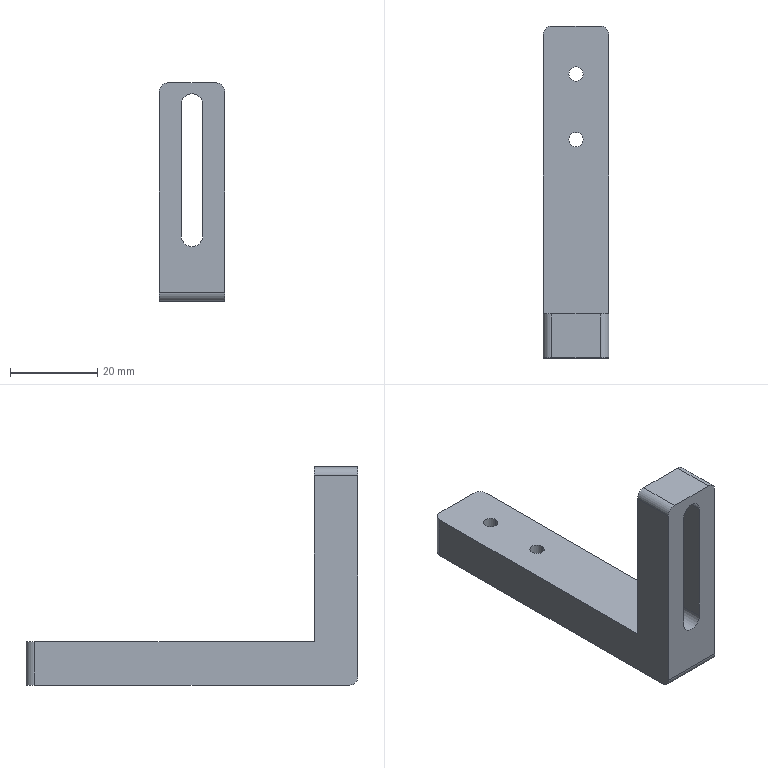Part | STEP file | 1004-2001-0086-1_1004-2001-0086-2 | 1 solid | 22 faces | box 15 x 76 x 50 mm | volume 15485 mm3 | cylinder 12 | plane 10 | commonest cylinder face diameters 4 x5 3.3 x4 5 x3
STEP:
#1=CARTESIAN_POINT('',(1.65,55.,-40.));
#2=VERTEX_POINT('',#1);
#3=CARTESIAN_POINT('',(-1.65,55.,-40.));
#4=VERTEX_POINT('',#3);
#5=CARTESIAN_POINT('',(0.,55.,-40.));
#6=DIRECTION('',(0.,0.,-1.));
#7=DIRECTION('',(-1.,0.,0.));
#8=AXIS2_PLACEMENT_3D('',#5,#6,#7);
#9=CIRCLE('',#8,1.65);
#10=EDGE_CURVE('',#2,#4,#9,.T.);
#11=ORIENTED_EDGE('',*,*,#10,.F.);
#12=CARTESIAN_POINT('',(1.65,55.,-50.));
#13=VERTEX_POINT('',#12);
#14=CARTESIAN_POINT('',(1.65,55.,-50.));
#15=DIRECTION('',(0.,0.,-1.));
#16=VECTOR('',#15,1000.);
#17=LINE('',#14,#16);
#18=EDGE_CURVE('',#2,#13,#17,.T.);
#19=ORIENTED_EDGE('',*,*,#18,.T.);
#20=CARTESIAN_POINT('',(-1.65,55.,-50.));
#21=VERTEX_POINT('',#20);
#22=CARTESIAN_POINT('',(0.,55.,-50.));
#23=DIRECTION('',(0.,0.,-1.));
#24=DIRECTION('',(-1.,0.,0.));
#25=AXIS2_PLACEMENT_3D('',#22,#23,#24);
#26=CIRCLE('',#25,1.65);
#27=EDGE_CURVE('',#13,#21,#26,.T.);
#28=ORIENTED_EDGE('',*,*,#27,.T.);
#29=CARTESIAN_POINT('',(-1.65,55.,-50.));
#30=DIRECTION('',(0.,0.,-1.));
#31=VECTOR('',#30,1000.);
#32=LINE('',#29,#31);
#33=EDGE_CURVE('',#4,#21,#32,.T.);
#34=ORIENTED_EDGE('',*,*,#33,.F.);
#35=EDGE_LOOP('',(#11,#19,#28,#34));
#36=FACE_OUTER_BOUND('',#35,.T.);
#37=CARTESIAN_POINT('',(0.,55.,-50.));
#38=DIRECTION('',(0.,0.,-1.));
#39=DIRECTION('',(-1.,0.,0.));
#40=AXIS2_PLACEMENT_3D('',#37,#38,#39);
#41=CYLINDRICAL_SURFACE('',#40,1.65);
#42=ADVANCED_FACE('',(#36),#41,.F.);
#43=CARTESIAN_POINT('',(1.65,40.,-40.));
#44=VERTEX_POINT('',#43);
#45=CARTESIAN_POINT('',(-1.65,40.,-40.));
#46=VERTEX_POINT('',#45);
#47=CARTESIAN_POINT('',(0.,40.,-40.));
#48=DIRECTION('',(0.,0.,-1.));
#49=DIRECTION('',(-1.,0.,0.));
#50=AXIS2_PLACEMENT_3D('',#47,#48,#49);
#51=CIRCLE('',#50,1.65);
#52=EDGE_CURVE('',#44,#46,#51,.T.);
#53=ORIENTED_EDGE('',*,*,#52,.F.);
#54=CARTESIAN_POINT('',(1.65,40.,-50.));
#55=VERTEX_POINT('',#54);
#56=CARTESIAN_POINT('',(1.65,40.,-50.));
#57=DIRECTION('',(0.,0.,-1.));
#58=VECTOR('',#57,1000.);
#59=LINE('',#56,#58);
#60=EDGE_CURVE('',#44,#55,#59,.T.);
#61=ORIENTED_EDGE('',*,*,#60,.T.);
#62=CARTESIAN_POINT('',(-1.65,40.,-50.));
#63=VERTEX_POINT('',#62);
#64=CARTESIAN_POINT('',(0.,40.,-50.));
#65=DIRECTION('',(0.,0.,-1.));
#66=DIRECTION('',(-1.,0.,0.));
#67=AXIS2_PLACEMENT_3D('',#64,#65,#66);
#68=CIRCLE('',#67,1.65);
#69=EDGE_CURVE('',#55,#63,#68,.T.);
#70=ORIENTED_EDGE('',*,*,#69,.T.);
#71=CARTESIAN_POINT('',(-1.65,40.,-50.));
#72=DIRECTION('',(0.,0.,-1.));
#73=VECTOR('',#72,1000.);
#74=LINE('',#71,#73);
#75=EDGE_CURVE('',#46,#63,#74,.T.);
#76=ORIENTED_EDGE('',*,*,#75,.F.);
#77=EDGE_LOOP('',(#53,#61,#70,#76));
#78=FACE_OUTER_BOUND('',#77,.T.);
#79=CARTESIAN_POINT('',(0.,40.,-50.));
#80=DIRECTION('',(0.,0.,-1.));
#81=DIRECTION('',(-1.,0.,0.));
#82=AXIS2_PLACEMENT_3D('',#79,#80,#81);
#83=CYLINDRICAL_SURFACE('',#82,1.65);
#84=ADVANCED_FACE('',(#78),#83,.F.);
#85=CARTESIAN_POINT('',(2.5,-10.,-5.));
#86=VERTEX_POINT('',#85);
#87=CARTESIAN_POINT('',(0.,-10.,-2.5));
#88=VERTEX_POINT('',#87);
#89=CARTESIAN_POINT('',(0.,-10.,-5.));
#90=DIRECTION('',(0.,-1.,0.));
#91=DIRECTION('',(0.,0.,1.));
#92=AXIS2_PLACEMENT_3D('',#89,#90,#91);
#93=CIRCLE('',#92,2.5);
#94=EDGE_CURVE('',#86,#88,#93,.T.);
#95=ORIENTED_EDGE('',*,*,#94,.T.);
#96=CARTESIAN_POINT('',(0.,0.,-2.5));
#97=VERTEX_POINT('',#96);
#98=CARTESIAN_POINT('',(0.,-10.,-2.5));
#99=DIRECTION('',(0.,1.,0.));
#100=VECTOR('',#99,1000.);
#101=LINE('',#98,#100);
#102=EDGE_CURVE('',#88,#97,#101,.T.);
#103=ORIENTED_EDGE('',*,*,#102,.T.);
#104=CARTESIAN_POINT('',(2.5,0.,-5.));
#105=VERTEX_POINT('',#104);
#106=CARTESIAN_POINT('',(0.,0.,-5.));
#107=DIRECTION('',(0.,-1.,0.));
#108=DIRECTION('',(0.,0.,1.));
#109=AXIS2_PLACEMENT_3D('',#106,#107,#108);
#110=CIRCLE('',#109,2.5);
#111=EDGE_CURVE('',#105,#97,#110,.T.);
#112=ORIENTED_EDGE('',*,*,#111,.F.);
#113=CARTESIAN_POINT('',(2.5,-10.,-5.));
#114=DIRECTION('',(0.,1.,0.));
#115=VECTOR('',#114,1000.);
#116=LINE('',#113,#115);
#117=EDGE_CURVE('',#86,#105,#116,.T.);
#118=ORIENTED_EDGE('',*,*,#117,.F.);
#119=EDGE_LOOP('',(#95,#103,#112,#118));
#120=FACE_OUTER_BOUND('',#119,.T.);
#121=CARTESIAN_POINT('',(0.,-10.,-5.));
#122=DIRECTION('',(0.,1.,0.));
#123=DIRECTION('',(0.,0.,1.));
#124=AXIS2_PLACEMENT_3D('',#121,#122,#123);
#125=CYLINDRICAL_SURFACE('',#124,2.5);
#126=ADVANCED_FACE('',(#120),#125,.F.);
#127=CARTESIAN_POINT('',(-7.5,64.,-40.));
#128=VERTEX_POINT('',#127);
#129=CARTESIAN_POINT('',(-7.5,64.,-50.));
#130=VERTEX_POINT('',#129);
#131=CARTESIAN_POINT('',(-7.5,64.,-50.));
#132=DIRECTION('',(0.,0.,-1.));
#133=VECTOR('',#132,1000.);
#134=LINE('',#131,#133);
#135=EDGE_CURVE('',#128,#130,#134,.T.);
#136=ORIENTED_EDGE('',*,*,#135,.T.);
#137=CARTESIAN_POINT('',(-7.5,-8.,-50.));
#138=VERTEX_POINT('',#137);
#139=CARTESIAN_POINT('',(-7.5,66.,-50.));
#140=DIRECTION('',(0.,-1.,0.));
#141=VECTOR('',#140,1000.);
#142=LINE('',#139,#141);
#143=EDGE_CURVE('',#130,#138,#142,.T.);
#144=ORIENTED_EDGE('',*,*,#143,.T.);
#145=CARTESIAN_POINT('',(-7.5,-10.,-48.));
#146=VERTEX_POINT('',#145);
#147=CARTESIAN_POINT('',(-7.5,-8.,-48.));
#148=DIRECTION('',(-1.,0.,0.));
#149=DIRECTION('',(0.,0.,1.));
#150=AXIS2_PLACEMENT_3D('',#147,#148,#149);
#151=CIRCLE('',#150,2.);
#152=EDGE_CURVE('',#138,#146,#151,.T.);
#153=ORIENTED_EDGE('',*,*,#152,.T.);
#154=CARTESIAN_POINT('',(-7.5,-10.,-2.));
#155=VERTEX_POINT('',#154);
#156=CARTESIAN_POINT('',(-7.5,-10.,-50.));
#157=DIRECTION('',(0.,0.,1.));
#158=VECTOR('',#157,1000.);
#159=LINE('',#156,#158);
#160=EDGE_CURVE('',#146,#155,#159,.T.);
#161=ORIENTED_EDGE('',*,*,#160,.T.);
#162=CARTESIAN_POINT('',(-7.5,0.,-2.));
#163=VERTEX_POINT('',#162);
#164=CARTESIAN_POINT('',(-7.5,66.,-2.));
#165=DIRECTION('',(0.,1.,0.));
#166=VECTOR('',#165,1000.);
#167=LINE('',#164,#166);
#168=EDGE_CURVE('',#155,#163,#167,.T.);
#169=ORIENTED_EDGE('',*,*,#168,.T.);
#170=CARTESIAN_POINT('',(-7.5,0.,-40.));
#171=VERTEX_POINT('',#170);
#172=CARTESIAN_POINT('',(-7.5,0.,-50.));
#173=DIRECTION('',(0.,0.,-1.));
#174=VECTOR('',#173,1000.);
#175=LINE('',#172,#174);
#176=EDGE_CURVE('',#163,#171,#175,.T.);
#177=ORIENTED_EDGE('',*,*,#176,.T.);
#178=CARTESIAN_POINT('',(-7.5,66.,-40.));
#179=DIRECTION('',(0.,1.,0.));
#180=VECTOR('',#179,1000.);
#181=LINE('',#178,#180);
#182=EDGE_CURVE('',#171,#128,#181,.T.);
#183=ORIENTED_EDGE('',*,*,#182,.T.);
#184=EDGE_LOOP('',(#136,#144,#153,#161,#169,#177,#183));
#185=FACE_OUTER_BOUND('',#184,.T.);
#186=CARTESIAN_POINT('',(-7.5,66.,-50.));
#187=DIRECTION('',(-1.,0.,0.));
#188=DIRECTION('',(0.,0.,1.));
#189=AXIS2_PLACEMENT_3D('',#186,#187,#188);
#190=PLANE('',#189);
#191=ADVANCED_FACE('',(#185),#190,.T.);
#192=CARTESIAN_POINT('',(0.,55.,-50.));
#193=DIRECTION('',(0.,0.,-1.));
#194=DIRECTION('',(-1.,0.,0.));
#195=AXIS2_PLACEMENT_3D('',#192,#193,#194);
#196=CIRCLE('',#195,1.65);
#197=EDGE_CURVE('',#21,#13,#196,.T.);
#198=ORIENTED_EDGE('',*,*,#197,.F.);
#199=ORIENTED_EDGE('',*,*,#27,.F.);
#200=EDGE_LOOP('',(#198,#199));
#201=FACE_BOUND('',#200,.T.);
#202=CARTESIAN_POINT('',(0.,40.,-50.));
#203=DIRECTION('',(0.,0.,-1.));
#204=DIRECTION('',(-1.,0.,0.));
#205=AXIS2_PLACEMENT_3D('',#202,#203,#204);
#206=CIRCLE('',#205,1.65);
#207=EDGE_CURVE('',#63,#55,#206,.T.);
#208=ORIENTED_EDGE('',*,*,#207,.F.);
#209=ORIENTED_EDGE('',*,*,#69,.F.);
#210=EDGE_LOOP('',(#208,#209));
#211=FACE_BOUND('',#210,.T.);
#212=ORIENTED_EDGE('',*,*,#143,.F.);
#213=CARTESIAN_POINT('',(-5.5,66.,-50.));
#214=VERTEX_POINT('',#213);
#215=CARTESIAN_POINT('',(-5.5,64.,-50.));
#216=DIRECTION('',(0.,0.,1.));
#217=DIRECTION('',(-1.,0.,0.));
#218=AXIS2_PLACEMENT_3D('',#215,#216,#217);
#219=CIRCLE('',#218,2.);
#220=EDGE_CURVE('',#214,#130,#219,.T.);
#221=ORIENTED_EDGE('',*,*,#220,.F.);
#222=CARTESIAN_POINT('',(5.5,66.,-50.));
#223=VERTEX_POINT('',#222);
#224=CARTESIAN_POINT('',(7.5,66.,-50.));
#225=DIRECTION('',(-1.,0.,0.));
#226=VECTOR('',#225,1000.);
#227=LINE('',#224,#226);
#228=EDGE_CURVE('',#223,#214,#227,.T.);
#229=ORIENTED_EDGE('',*,*,#228,.F.);
#230=CARTESIAN_POINT('',(7.5,64.,-50.));
#231=VERTEX_POINT('',#230);
#232=CARTESIAN_POINT('',(5.5,64.,-50.));
#233=DIRECTION('',(0.,0.,1.));
#234=DIRECTION('',(1.,0.,0.));
#235=AXIS2_PLACEMENT_3D('',#232,#233,#234);
#236=CIRCLE('',#235,2.);
#237=EDGE_CURVE('',#231,#223,#236,.T.);
#238=ORIENTED_EDGE('',*,*,#237,.F.);
#239=CARTESIAN_POINT('',(7.5,-8.,-50.));
#240=VERTEX_POINT('',#239);
#241=CARTESIAN_POINT('',(7.5,0.,-50.));
#242=DIRECTION('',(0.,1.,0.));
#243=VECTOR('',#242,1000.);
#244=LINE('',#241,#243);
#245=EDGE_CURVE('',#240,#231,#244,.T.);
#246=ORIENTED_EDGE('',*,*,#245,.F.);
#247=CARTESIAN_POINT('',(7.5,-8.,-50.));
#248=DIRECTION('',(1.,0.,0.));
#249=VECTOR('',#248,1000.);
#250=LINE('',#247,#249);
#251=EDGE_CURVE('',#138,#240,#250,.T.);
#252=ORIENTED_EDGE('',*,*,#251,.F.);
#253=EDGE_LOOP('',(#212,#221,#229,#238,#246,#252));
#254=FACE_OUTER_BOUND('',#253,.T.);
#255=CARTESIAN_POINT('',(7.5,0.,-50.));
#256=DIRECTION('',(0.,0.,1.));
#257=DIRECTION('',(1.,0.,0.));
#258=AXIS2_PLACEMENT_3D('',#255,#256,#257);
#259=PLANE('',#258);
#260=ADVANCED_FACE('',(#201,#211,#254),#259,.F.);
#261=ORIENTED_EDGE('',*,*,#135,.F.);
#262=CARTESIAN_POINT('',(-5.5,66.,-40.));
#263=VERTEX_POINT('',#262);
#264=CARTESIAN_POINT('',(-5.5,64.,-40.));
#265=DIRECTION('',(0.,0.,-1.));
#266=DIRECTION('',(-1.,0.,0.));
#267=AXIS2_PLACEMENT_3D('',#264,#265,#266);
#268=CIRCLE('',#267,2.);
#269=EDGE_CURVE('',#128,#263,#268,.T.);
#270=ORIENTED_EDGE('',*,*,#269,.T.);
#271=CARTESIAN_POINT('',(-5.5,66.,-50.));
#272=DIRECTION('',(0.,0.,-1.));
#273=VECTOR('',#272,1000.);
#274=LINE('',#271,#273);
#275=EDGE_CURVE('',#263,#214,#274,.T.);
#276=ORIENTED_EDGE('',*,*,#275,.T.);
#277=ORIENTED_EDGE('',*,*,#220,.T.);
#278=EDGE_LOOP('',(#261,#270,#276,#277));
#279=FACE_OUTER_BOUND('',#278,.T.);
#280=CARTESIAN_POINT('',(-5.5,64.,-50.));
#281=DIRECTION('',(0.,0.,-1.));
#282=DIRECTION('',(-1.,0.,0.));
#283=AXIS2_PLACEMENT_3D('',#280,#281,#282);
#284=CYLINDRICAL_SURFACE('',#283,2.);
#285=ADVANCED_FACE('',(#279),#284,.T.);
#286=CARTESIAN_POINT('',(0.,55.,-40.));
#287=DIRECTION('',(0.,0.,-1.));
#288=DIRECTION('',(-1.,0.,0.));
#289=AXIS2_PLACEMENT_3D('',#286,#287,#288);
#290=CIRCLE('',#289,1.65);
#291=EDGE_CURVE('',#4,#2,#290,.T.);
#292=ORIENTED_EDGE('',*,*,#291,.T.);
#293=ORIENTED_EDGE('',*,*,#10,.T.);
#294=EDGE_LOOP('',(#292,#293));
#295=FACE_BOUND('',#294,.T.);
#296=CARTESIAN_POINT('',(0.,40.,-40.));
#297=DIRECTION('',(0.,0.,-1.));
#298=DIRECTION('',(-1.,0.,0.));
#299=AXIS2_PLACEMENT_3D('',#296,#297,#298);
#300=CIRCLE('',#299,1.65);
#301=EDGE_CURVE('',#46,#44,#300,.T.);
#302=ORIENTED_EDGE('',*,*,#301,.T.);
#303=ORIENTED_EDGE('',*,*,#52,.T.);
#304=EDGE_LOOP('',(#302,#303));
#305=FACE_BOUND('',#304,.T.);
#306=CARTESIAN_POINT('',(7.5,64.,-40.));
#307=VERTEX_POINT('',#306);
#308=CARTESIAN_POINT('',(5.5,66.,-40.));
#309=VERTEX_POINT('',#308);
#310=CARTESIAN_POINT('',(5.5,64.,-40.));
#311=DIRECTION('',(0.,0.,1.));
#312=DIRECTION('',(1.,0.,0.));
#313=AXIS2_PLACEMENT_3D('',#310,#311,#312);
#314=CIRCLE('',#313,2.);
#315=EDGE_CURVE('',#307,#309,#314,.T.);
#316=ORIENTED_EDGE('',*,*,#315,.T.);
#317=CARTESIAN_POINT('',(7.5,66.,-40.));
#318=DIRECTION('',(-1.,0.,0.));
#319=VECTOR('',#318,1000.);
#320=LINE('',#317,#319);
#321=EDGE_CURVE('',#309,#263,#320,.T.);
#322=ORIENTED_EDGE('',*,*,#321,.T.);
#323=ORIENTED_EDGE('',*,*,#269,.F.);
#324=ORIENTED_EDGE('',*,*,#182,.F.);
#325=CARTESIAN_POINT('',(7.5,0.,-40.));
#326=VERTEX_POINT('',#325);
#327=CARTESIAN_POINT('',(7.5,0.,-40.));
#328=DIRECTION('',(1.,0.,0.));
#329=VECTOR('',#328,1000.);
#330=LINE('',#327,#329);
#331=EDGE_CURVE('',#171,#326,#330,.T.);
#332=ORIENTED_EDGE('',*,*,#331,.T.);
#333=CARTESIAN_POINT('',(7.5,0.,-40.));
#334=DIRECTION('',(0.,1.,0.));
#335=VECTOR('',#334,1000.);
#336=LINE('',#333,#335);
#337=EDGE_CURVE('',#326,#307,#336,.T.);
#338=ORIENTED_EDGE('',*,*,#337,.T.);
#339=EDGE_LOOP('',(#316,#322,#323,#324,#332,#338));
#340=FACE_OUTER_BOUND('',#339,.T.);
#341=CARTESIAN_POINT('',(7.5,0.,-40.));
#342=DIRECTION('',(0.,0.,1.));
#343=DIRECTION('',(1.,0.,0.));
#344=AXIS2_PLACEMENT_3D('',#341,#342,#343);
#345=PLANE('',#344);
#346=ADVANCED_FACE('',(#295,#305,#340),#345,.T.);
#347=CARTESIAN_POINT('',(-2.5,0.,-5.));
#348=VERTEX_POINT('',#347);
#349=CARTESIAN_POINT('',(-2.5,0.,-35.));
#350=VERTEX_POINT('',#349);
#351=CARTESIAN_POINT('',(-2.5,0.,0.));
#352=DIRECTION('',(0.,0.,-1.));
#353=VECTOR('',#352,1000.);
#354=LINE('',#351,#353);
#355=EDGE_CURVE('',#348,#350,#354,.T.);
#356=ORIENTED_EDGE('',*,*,#355,.T.);
#357=CARTESIAN_POINT('',(2.5,0.,-35.));
#358=VERTEX_POINT('',#357);
#359=CARTESIAN_POINT('',(0.,0.,-35.));
#360=DIRECTION('',(0.,-1.,0.));
#361=DIRECTION('',(0.,0.,1.));
#362=AXIS2_PLACEMENT_3D('',#359,#360,#361);
#363=CIRCLE('',#362,2.5);
#364=EDGE_CURVE('',#350,#358,#363,.T.);
#365=ORIENTED_EDGE('',*,*,#364,.T.);
#366=CARTESIAN_POINT('',(2.5,0.,0.));
#367=DIRECTION('',(0.,0.,1.));
#368=VECTOR('',#367,1000.);
#369=LINE('',#366,#368);
#370=EDGE_CURVE('',#358,#105,#369,.T.);
#371=ORIENTED_EDGE('',*,*,#370,.T.);
#372=ORIENTED_EDGE('',*,*,#111,.T.);
#373=CARTESIAN_POINT('',(0.,0.,-5.));
#374=DIRECTION('',(0.,-1.,0.));
#375=DIRECTION('',(0.,0.,1.));
#376=AXIS2_PLACEMENT_3D('',#373,#374,#375);
#377=CIRCLE('',#376,2.5);
#378=EDGE_CURVE('',#97,#348,#377,.T.);
#379=ORIENTED_EDGE('',*,*,#378,.T.);
#380=EDGE_LOOP('',(#356,#365,#371,#372,#379));
#381=FACE_BOUND('',#380,.T.);
#382=ORIENTED_EDGE('',*,*,#331,.F.);
#383=ORIENTED_EDGE('',*,*,#176,.F.);
#384=CARTESIAN_POINT('',(-5.5,0.,0.));
#385=VERTEX_POINT('',#384);
#386=CARTESIAN_POINT('',(-5.5,0.,-2.));
#387=DIRECTION('',(0.,1.,0.));
#388=DIRECTION('',(0.,0.,1.));
#389=AXIS2_PLACEMENT_3D('',#386,#387,#388);
#390=CIRCLE('',#389,2.);
#391=EDGE_CURVE('',#163,#385,#390,.T.);
#392=ORIENTED_EDGE('',*,*,#391,.T.);
#393=CARTESIAN_POINT('',(5.5,0.,0.));
#394=VERTEX_POINT('',#393);
#395=CARTESIAN_POINT('',(7.5,0.,0.));
#396=DIRECTION('',(1.,0.,0.));
#397=VECTOR('',#396,1000.);
#398=LINE('',#395,#397);
#399=EDGE_CURVE('',#385,#394,#398,.T.);
#400=ORIENTED_EDGE('',*,*,#399,.T.);
#401=CARTESIAN_POINT('',(7.5,0.,-2.));
#402=VERTEX_POINT('',#401);
#403=CARTESIAN_POINT('',(5.5,0.,-2.));
#404=DIRECTION('',(0.,1.,0.));
#405=DIRECTION('',(0.,0.,-1.));
#406=AXIS2_PLACEMENT_3D('',#403,#404,#405);
#407=CIRCLE('',#406,2.);
#408=EDGE_CURVE('',#394,#402,#407,.T.);
#409=ORIENTED_EDGE('',*,*,#408,.T.);
#410=CARTESIAN_POINT('',(7.5,0.,0.));
#411=DIRECTION('',(0.,0.,-1.));
#412=VECTOR('',#411,1000.);
#413=LINE('',#410,#412);
#414=EDGE_CURVE('',#402,#326,#413,.T.);
#415=ORIENTED_EDGE('',*,*,#414,.T.);
#416=EDGE_LOOP('',(#382,#383,#392,#400,#409,#415));
#417=FACE_OUTER_BOUND('',#416,.T.);
#418=CARTESIAN_POINT('',(7.5,0.,0.));
#419=DIRECTION('',(0.,1.,0.));
#420=DIRECTION('',(0.,0.,1.));
#421=AXIS2_PLACEMENT_3D('',#418,#419,#420);
#422=PLANE('',#421);
#423=ADVANCED_FACE('',(#381,#417),#422,.T.);
#424=ORIENTED_EDGE('',*,*,#168,.F.);
#425=CARTESIAN_POINT('',(-5.5,-10.,0.));
#426=VERTEX_POINT('',#425);
#427=CARTESIAN_POINT('',(-5.5,-10.,-2.));
#428=DIRECTION('',(0.,1.,0.));
#429=DIRECTION('',(0.,0.,1.));
#430=AXIS2_PLACEMENT_3D('',#427,#428,#429);
#431=CIRCLE('',#430,2.);
#432=EDGE_CURVE('',#155,#426,#431,.T.);
#433=ORIENTED_EDGE('',*,*,#432,.T.);
#434=CARTESIAN_POINT('',(-5.5,66.,0.));
#435=DIRECTION('',(0.,1.,0.));
#436=VECTOR('',#435,1000.);
#437=LINE('',#434,#436);
#438=EDGE_CURVE('',#426,#385,#437,.T.);
#439=ORIENTED_EDGE('',*,*,#438,.T.);
#440=ORIENTED_EDGE('',*,*,#391,.F.);
#441=EDGE_LOOP('',(#424,#433,#439,#440));
#442=FACE_OUTER_BOUND('',#441,.T.);
#443=CARTESIAN_POINT('',(-5.5,66.,-2.));
#444=DIRECTION('',(0.,1.,0.));
#445=DIRECTION('',(0.,0.,1.));
#446=AXIS2_PLACEMENT_3D('',#443,#444,#445);
#447=CYLINDRICAL_SURFACE('',#446,2.);
#448=ADVANCED_FACE('',(#442),#447,.T.);
#449=CARTESIAN_POINT('',(-2.5,-10.,-35.));
#450=VERTEX_POINT('',#449);
#451=CARTESIAN_POINT('',(2.5,-10.,-35.));
#452=VERTEX_POINT('',#451);
#453=CARTESIAN_POINT('',(0.,-10.,-35.));
#454=DIRECTION('',(0.,-1.,0.));
#455=DIRECTION('',(0.,0.,1.));
#456=AXIS2_PLACEMENT_3D('',#453,#454,#455);
#457=CIRCLE('',#456,2.5);
#458=EDGE_CURVE('',#450,#452,#457,.T.);
#459=ORIENTED_EDGE('',*,*,#458,.F.);
#460=CARTESIAN_POINT('',(-2.5,-10.,-5.));
#461=VERTEX_POINT('',#460);
#462=CARTESIAN_POINT('',(-2.5,-10.,0.));
#463=DIRECTION('',(0.,0.,-1.));
#464=VECTOR('',#463,1000.);
#465=LINE('',#462,#464);
#466=EDGE_CURVE('',#461,#450,#465,.T.);
#467=ORIENTED_EDGE('',*,*,#466,.F.);
#468=CARTESIAN_POINT('',(0.,-10.,-5.));
#469=DIRECTION('',(0.,-1.,0.));
#470=DIRECTION('',(0.,0.,1.));
#471=AXIS2_PLACEMENT_3D('',#468,#469,#470);
#472=CIRCLE('',#471,2.5);
#473=EDGE_CURVE('',#88,#461,#472,.T.);
#474=ORIENTED_EDGE('',*,*,#473,.F.);
#475=ORIENTED_EDGE('',*,*,#94,.F.);
#476=CARTESIAN_POINT('',(2.5,-10.,0.));
#477=DIRECTION('',(0.,0.,1.));
#478=VECTOR('',#477,1000.);
#479=LINE('',#476,#478);
#480=EDGE_CURVE('',#452,#86,#479,.T.);
#481=ORIENTED_EDGE('',*,*,#480,.F.);
#482=EDGE_LOOP('',(#459,#467,#474,#475,#481));
#483=FACE_BOUND('',#482,.T.);
#484=CARTESIAN_POINT('',(7.5,-10.,-2.));
#485=VERTEX_POINT('',#484);
#486=CARTESIAN_POINT('',(7.5,-10.,-48.));
#487=VERTEX_POINT('',#486);
#488=CARTESIAN_POINT('',(7.5,-10.,0.));
#489=DIRECTION('',(0.,0.,-1.));
#490=VECTOR('',#489,1000.);
#491=LINE('',#488,#490);
#492=EDGE_CURVE('',#485,#487,#491,.T.);
#493=ORIENTED_EDGE('',*,*,#492,.F.);
#494=CARTESIAN_POINT('',(5.5,-10.,0.));
#495=VERTEX_POINT('',#494);
#496=CARTESIAN_POINT('',(5.5,-10.,-2.));
#497=DIRECTION('',(0.,1.,0.));
#498=DIRECTION('',(0.,0.,-1.));
#499=AXIS2_PLACEMENT_3D('',#496,#497,#498);
#500=CIRCLE('',#499,2.);
#501=EDGE_CURVE('',#495,#485,#500,.T.);
#502=ORIENTED_EDGE('',*,*,#501,.F.);
#503=CARTESIAN_POINT('',(7.5,-10.,0.));
#504=DIRECTION('',(1.,0.,0.));
#505=VECTOR('',#504,1000.);
#506=LINE('',#503,#505);
#507=EDGE_CURVE('',#426,#495,#506,.T.);
#508=ORIENTED_EDGE('',*,*,#507,.F.);
#509=ORIENTED_EDGE('',*,*,#432,.F.);
#510=ORIENTED_EDGE('',*,*,#160,.F.);
#511=CARTESIAN_POINT('',(7.5,-10.,-48.));
#512=DIRECTION('',(-1.,0.,0.));
#513=VECTOR('',#512,1000.);
#514=LINE('',#511,#513);
#515=EDGE_CURVE('',#487,#146,#514,.T.);
#516=ORIENTED_EDGE('',*,*,#515,.F.);
#517=EDGE_LOOP('',(#493,#502,#508,#509,#510,#516));
#518=FACE_OUTER_BOUND('',#517,.T.);
#519=CARTESIAN_POINT('',(7.5,-10.,0.));
#520=DIRECTION('',(0.,1.,0.));
#521=DIRECTION('',(0.,0.,1.));
#522=AXIS2_PLACEMENT_3D('',#519,#520,#521);
#523=PLANE('',#522);
#524=ADVANCED_FACE('',(#483,#518),#523,.F.);
#525=ORIENTED_EDGE('',*,*,#251,.T.);
#526=CARTESIAN_POINT('',(7.5,-8.,-48.));
#527=DIRECTION('',(-1.,0.,0.));
#528=DIRECTION('',(0.,0.,1.));
#529=AXIS2_PLACEMENT_3D('',#526,#527,#528);
#530=CIRCLE('',#529,2.);
#531=EDGE_CURVE('',#240,#487,#530,.T.);
#532=ORIENTED_EDGE('',*,*,#531,.T.);
#533=ORIENTED_EDGE('',*,*,#515,.T.);
#534=ORIENTED_EDGE('',*,*,#152,.F.);
#535=EDGE_LOOP('',(#525,#532,#533,#534));
#536=FACE_OUTER_BOUND('',#535,.T.);
#537=CARTESIAN_POINT('',(7.5,-8.,-48.));
#538=DIRECTION('',(-1.,0.,0.));
#539=DIRECTION('',(0.,0.,1.));
#540=AXIS2_PLACEMENT_3D('',#537,#538,#539);
#541=CYLINDRICAL_SURFACE('',#540,2.);
#542=ADVANCED_FACE('',(#536),#541,.T.);
#543=ORIENTED_EDGE('',*,*,#18,.F.);
#544=ORIENTED_EDGE('',*,*,#291,.F.);
#545=ORIENTED_EDGE('',*,*,#33,.T.);
#546=ORIENTED_EDGE('',*,*,#197,.T.);
#547=EDGE_LOOP('',(#543,#544,#545,#546));
#548=FACE_OUTER_BOUND('',#547,.T.);
#549=CARTESIAN_POINT('',(0.,55.,-50.));
#550=DIRECTION('',(0.,0.,-1.));
#551=DIRECTION('',(-1.,0.,0.));
#552=AXIS2_PLACEMENT_3D('',#549,#550,#551);
#553=CYLINDRICAL_SURFACE('',#552,1.65);
#554=ADVANCED_FACE('',(#548),#553,.F.);
#555=ORIENTED_EDGE('',*,*,#60,.F.);
#556=ORIENTED_EDGE('',*,*,#301,.F.);
#557=ORIENTED_EDGE('',*,*,#75,.T.);
#558=ORIENTED_EDGE('',*,*,#207,.T.);
#559=EDGE_LOOP('',(#555,#556,#557,#558));
#560=FACE_OUTER_BOUND('',#559,.T.);
#561=CARTESIAN_POINT('',(0.,40.,-50.));
#562=DIRECTION('',(0.,0.,-1.));
#563=DIRECTION('',(-1.,0.,0.));
#564=AXIS2_PLACEMENT_3D('',#561,#562,#563);
#565=CYLINDRICAL_SURFACE('',#564,1.65);
#566=ADVANCED_FACE('',(#560),#565,.F.);
#567=CARTESIAN_POINT('',(5.5,66.,-40.));
#568=DIRECTION('',(0.,0.,-1.));
#569=VECTOR('',#568,1000.);
#570=LINE('',#567,#569);
#571=EDGE_CURVE('',#309,#223,#570,.T.);
#572=ORIENTED_EDGE('',*,*,#571,.T.);
#573=ORIENTED_EDGE('',*,*,#228,.T.);
#574=ORIENTED_EDGE('',*,*,#275,.F.);
#575=ORIENTED_EDGE('',*,*,#321,.F.);
#576=EDGE_LOOP('',(#572,#573,#574,#575));
#577=FACE_OUTER_BOUND('',#576,.T.);
#578=CARTESIAN_POINT('',(7.5,66.,-40.));
#579=DIRECTION('',(0.,1.,0.));
#580=DIRECTION('',(0.,0.,1.));
#581=AXIS2_PLACEMENT_3D('',#578,#579,#580);
#582=PLANE('',#581);
#583=ADVANCED_FACE('',(#577),#582,.T.);
#584=ORIENTED_EDGE('',*,*,#571,.F.);
#585=ORIENTED_EDGE('',*,*,#315,.F.);
#586=CARTESIAN_POINT('',(7.5,64.,-40.));
#587=DIRECTION('',(0.,0.,-1.));
#588=VECTOR('',#587,1000.);
#589=LINE('',#586,#588);
#590=EDGE_CURVE('',#307,#231,#589,.T.);
#591=ORIENTED_EDGE('',*,*,#590,.T.);
#592=ORIENTED_EDGE('',*,*,#237,.T.);
#593=EDGE_LOOP('',(#584,#585,#591,#592));
#594=FACE_OUTER_BOUND('',#593,.T.);
#595=CARTESIAN_POINT('',(5.5,64.,-40.));
#596=DIRECTION('',(0.,0.,1.));
#597=DIRECTION('',(1.,0.,0.));
#598=AXIS2_PLACEMENT_3D('',#595,#596,#597);
#599=CYLINDRICAL_SURFACE('',#598,2.);
#600=ADVANCED_FACE('',(#594),#599,.T.);
#601=ORIENTED_EDGE('',*,*,#245,.T.);
#602=ORIENTED_EDGE('',*,*,#590,.F.);
#603=ORIENTED_EDGE('',*,*,#337,.F.);
#604=ORIENTED_EDGE('',*,*,#414,.F.);
#605=CARTESIAN_POINT('',(7.5,66.,-2.));
#606=DIRECTION('',(0.,1.,0.));
#607=VECTOR('',#606,1000.);
#608=LINE('',#605,#607);
#609=EDGE_CURVE('',#485,#402,#608,.T.);
#610=ORIENTED_EDGE('',*,*,#609,.F.);
#611=ORIENTED_EDGE('',*,*,#492,.T.);
#612=ORIENTED_EDGE('',*,*,#531,.F.);
#613=EDGE_LOOP('',(#601,#602,#603,#604,#610,#611,#612));
#614=FACE_OUTER_BOUND('',#613,.T.);
#615=CARTESIAN_POINT('',(7.5,66.,-50.));
#616=DIRECTION('',(-1.,0.,0.));
#617=DIRECTION('',(0.,0.,1.));
#618=AXIS2_PLACEMENT_3D('',#615,#616,#617);
#619=PLANE('',#618);
#620=ADVANCED_FACE('',(#614),#619,.F.);
#621=CARTESIAN_POINT('',(-2.5,-10.,-35.));
#622=DIRECTION('',(0.,1.,0.));
#623=VECTOR('',#622,1000.);
#624=LINE('',#621,#623);
#625=EDGE_CURVE('',#450,#350,#624,.T.);
#626=ORIENTED_EDGE('',*,*,#625,.F.);
#627=ORIENTED_EDGE('',*,*,#458,.T.);
#628=CARTESIAN_POINT('',(2.5,-10.,-35.));
#629=DIRECTION('',(0.,-1.,0.));
#630=VECTOR('',#629,1000.);
#631=LINE('',#628,#630);
#632=EDGE_CURVE('',#358,#452,#631,.T.);
#633=ORIENTED_EDGE('',*,*,#632,.F.);
#634=ORIENTED_EDGE('',*,*,#364,.F.);
#635=EDGE_LOOP('',(#626,#627,#633,#634));
#636=FACE_OUTER_BOUND('',#635,.T.);
#637=CARTESIAN_POINT('',(0.,-10.,-35.));
#638=DIRECTION('',(0.,1.,0.));
#639=DIRECTION('',(0.,0.,1.));
#640=AXIS2_PLACEMENT_3D('',#637,#638,#639);
#641=CYLINDRICAL_SURFACE('',#640,2.5);
#642=ADVANCED_FACE('',(#636),#641,.F.);
#643=ORIENTED_EDGE('',*,*,#466,.T.);
#644=ORIENTED_EDGE('',*,*,#625,.T.);
#645=ORIENTED_EDGE('',*,*,#355,.F.);
#646=CARTESIAN_POINT('',(-2.5,-10.,-5.));
#647=DIRECTION('',(0.,1.,0.));
#648=VECTOR('',#647,1000.);
#649=LINE('',#646,#648);
#650=EDGE_CURVE('',#461,#348,#649,.T.);
#651=ORIENTED_EDGE('',*,*,#650,.F.);
#652=EDGE_LOOP('',(#643,#644,#645,#651));
#653=FACE_OUTER_BOUND('',#652,.T.);
#654=CARTESIAN_POINT('',(-2.5,-10.,-35.));
#655=DIRECTION('',(-1.,0.,0.));
#656=DIRECTION('',(0.,0.,1.));
#657=AXIS2_PLACEMENT_3D('',#654,#655,#656);
#658=PLANE('',#657);
#659=ADVANCED_FACE('',(#653),#658,.F.);
#660=ORIENTED_EDGE('',*,*,#102,.F.);
#661=ORIENTED_EDGE('',*,*,#473,.T.);
#662=ORIENTED_EDGE('',*,*,#650,.T.);
#663=ORIENTED_EDGE('',*,*,#378,.F.);
#664=EDGE_LOOP('',(#660,#661,#662,#663));
#665=FACE_OUTER_BOUND('',#664,.T.);
#666=CARTESIAN_POINT('',(0.,-10.,-5.));
#667=DIRECTION('',(0.,1.,0.));
#668=DIRECTION('',(0.,0.,1.));
#669=AXIS2_PLACEMENT_3D('',#666,#667,#668);
#670=CYLINDRICAL_SURFACE('',#669,2.5);
#671=ADVANCED_FACE('',(#665),#670,.F.);
#672=ORIENTED_EDGE('',*,*,#480,.T.);
#673=ORIENTED_EDGE('',*,*,#117,.T.);
#674=ORIENTED_EDGE('',*,*,#370,.F.);
#675=ORIENTED_EDGE('',*,*,#632,.T.);
#676=EDGE_LOOP('',(#672,#673,#674,#675));
#677=FACE_OUTER_BOUND('',#676,.T.);
#678=CARTESIAN_POINT('',(2.5,-10.,-35.));
#679=DIRECTION('',(1.,0.,0.));
#680=DIRECTION('',(0.,0.,-1.));
#681=AXIS2_PLACEMENT_3D('',#678,#679,#680);
#682=PLANE('',#681);
#683=ADVANCED_FACE('',(#677),#682,.F.);
#684=CARTESIAN_POINT('',(5.5,-10.,0.));
#685=DIRECTION('',(0.,-1.,0.));
#686=VECTOR('',#685,1000.);
#687=LINE('',#684,#686);
#688=EDGE_CURVE('',#394,#495,#687,.T.);
#689=ORIENTED_EDGE('',*,*,#688,.T.);
#690=ORIENTED_EDGE('',*,*,#501,.T.);
#691=ORIENTED_EDGE('',*,*,#609,.T.);
#692=ORIENTED_EDGE('',*,*,#408,.F.);
#693=EDGE_LOOP('',(#689,#690,#691,#692));
#694=FACE_OUTER_BOUND('',#693,.T.);
#695=CARTESIAN_POINT('',(5.5,-10.,-2.));
#696=DIRECTION('',(0.,-1.,0.));
#697=DIRECTION('',(0.,0.,-1.));
#698=AXIS2_PLACEMENT_3D('',#695,#696,#697);
#699=CYLINDRICAL_SURFACE('',#698,2.);
#700=ADVANCED_FACE('',(#694),#699,.T.);
#701=ORIENTED_EDGE('',*,*,#688,.F.);
#702=ORIENTED_EDGE('',*,*,#399,.F.);
#703=ORIENTED_EDGE('',*,*,#438,.F.);
#704=ORIENTED_EDGE('',*,*,#507,.T.);
#705=EDGE_LOOP('',(#701,#702,#703,#704));
#706=FACE_OUTER_BOUND('',#705,.T.);
#707=CARTESIAN_POINT('',(7.5,-10.,0.));
#708=DIRECTION('',(0.,0.,1.));
#709=DIRECTION('',(1.,0.,0.));
#710=AXIS2_PLACEMENT_3D('',#707,#708,#709);
#711=PLANE('',#710);
#712=ADVANCED_FACE('',(#706),#711,.T.);
#713=CLOSED_SHELL('',(#42,#84,#126,#191,#260,#285,#346,#423,#448,#524,#542,#554,#566,#583,#600,#620,#642,#659,#671,#683,#700,#712));
#714=MANIFOLD_SOLID_BREP('',#713);
#715=CARTESIAN_POINT('',(0.,0.,0.));
#716=DIRECTION('',(0.,0.,1.));
#717=DIRECTION('',(1.,0.,0.));
#718=AXIS2_PLACEMENT_3D('',#715,#716,#717);
#719=(LENGTH_UNIT()NAMED_UNIT(*)SI_UNIT(.MILLI.,.METRE.));
#720=UNCERTAINTY_MEASURE_WITH_UNIT(LENGTH_MEASURE(0.00001),#719,'','');
#721=(NAMED_UNIT(*)PLANE_ANGLE_UNIT()SI_UNIT($,.RADIAN.));
#722=(NAMED_UNIT(*)SI_UNIT($,.STERADIAN.)SOLID_ANGLE_UNIT());
#723=(GEOMETRIC_REPRESENTATION_CONTEXT(3)GLOBAL_UNCERTAINTY_ASSIGNED_CONTEXT((#720))GLOBAL_UNIT_ASSIGNED_CONTEXT((#719,#721,#722))REPRESENTATION_CONTEXT('',''));
#724=ADVANCED_BREP_SHAPE_REPRESENTATION('',(#714,#718),#723);